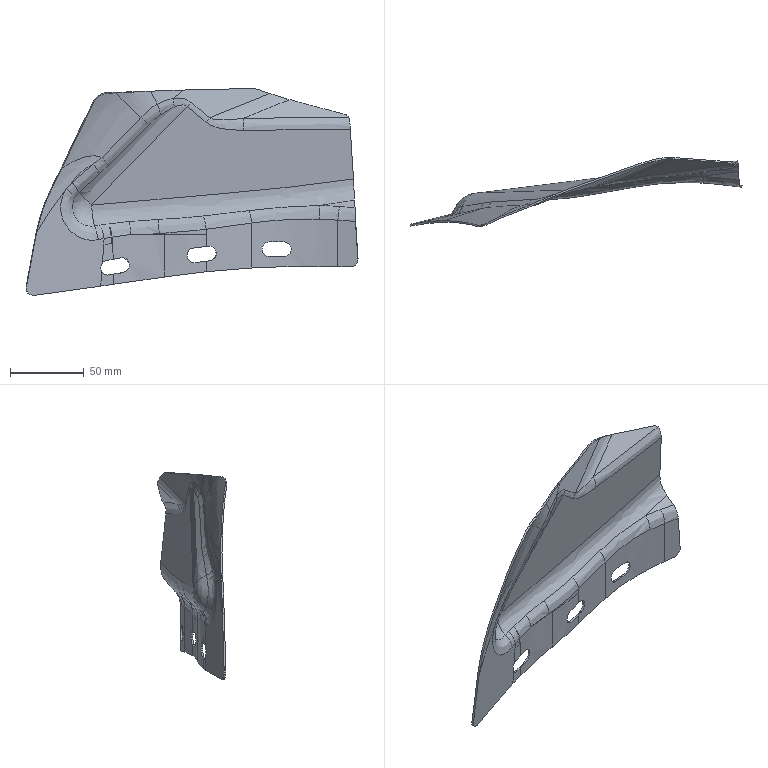Part | STEP file | FNA5401731 | 1 solid | 150 faces | box 225.797 x 47.255 x 140.75 mm | volume 31228 mm3 | spline 120 | plane 19 | cylinder 6 | other 3 | torus 2 | commonest cylinder face diameters 36.2 x1 38.6 x1 396.2 x1 398.6 x1 440.2 x1 442.6 x1